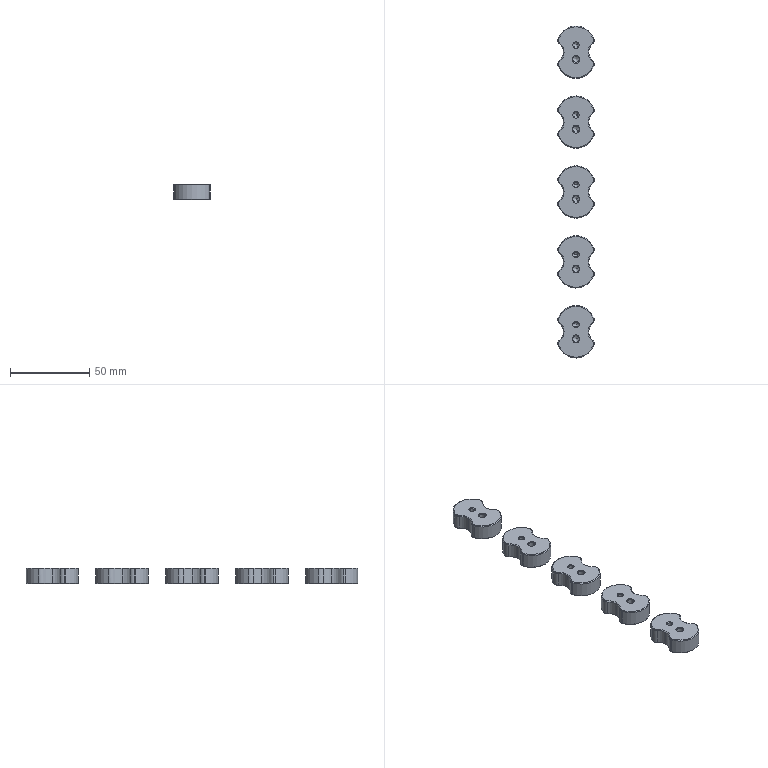Part | 5 solids | 235 faces | box 22.923 x 209 x 10 mm | volume 28792 mm3 | cone 150 | cylinder 75 | plane 10 | commonest cylinder face diameters 6 x30 14 x15 3 x10 4 x10 24 x10